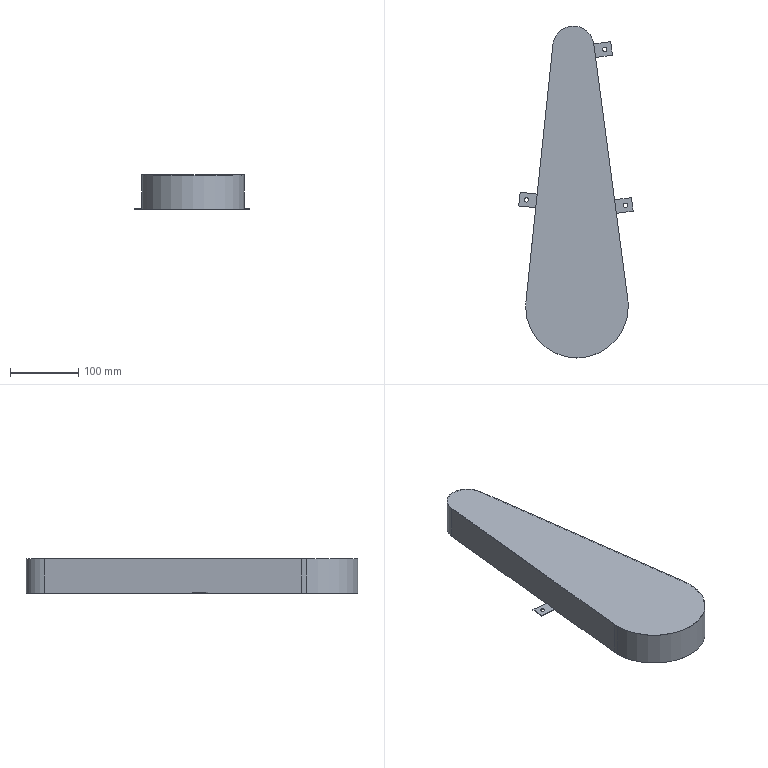Part | STEP file | Protective cover | 1 solid | 33 faces | box 167.34 x 485.19 x 50 mm | volume 105387 mm3 | plane 19 | cylinder 14 | commonest cylinder face diameters 6.5 x6 148 x3 150 x3 58 x1 60 x1